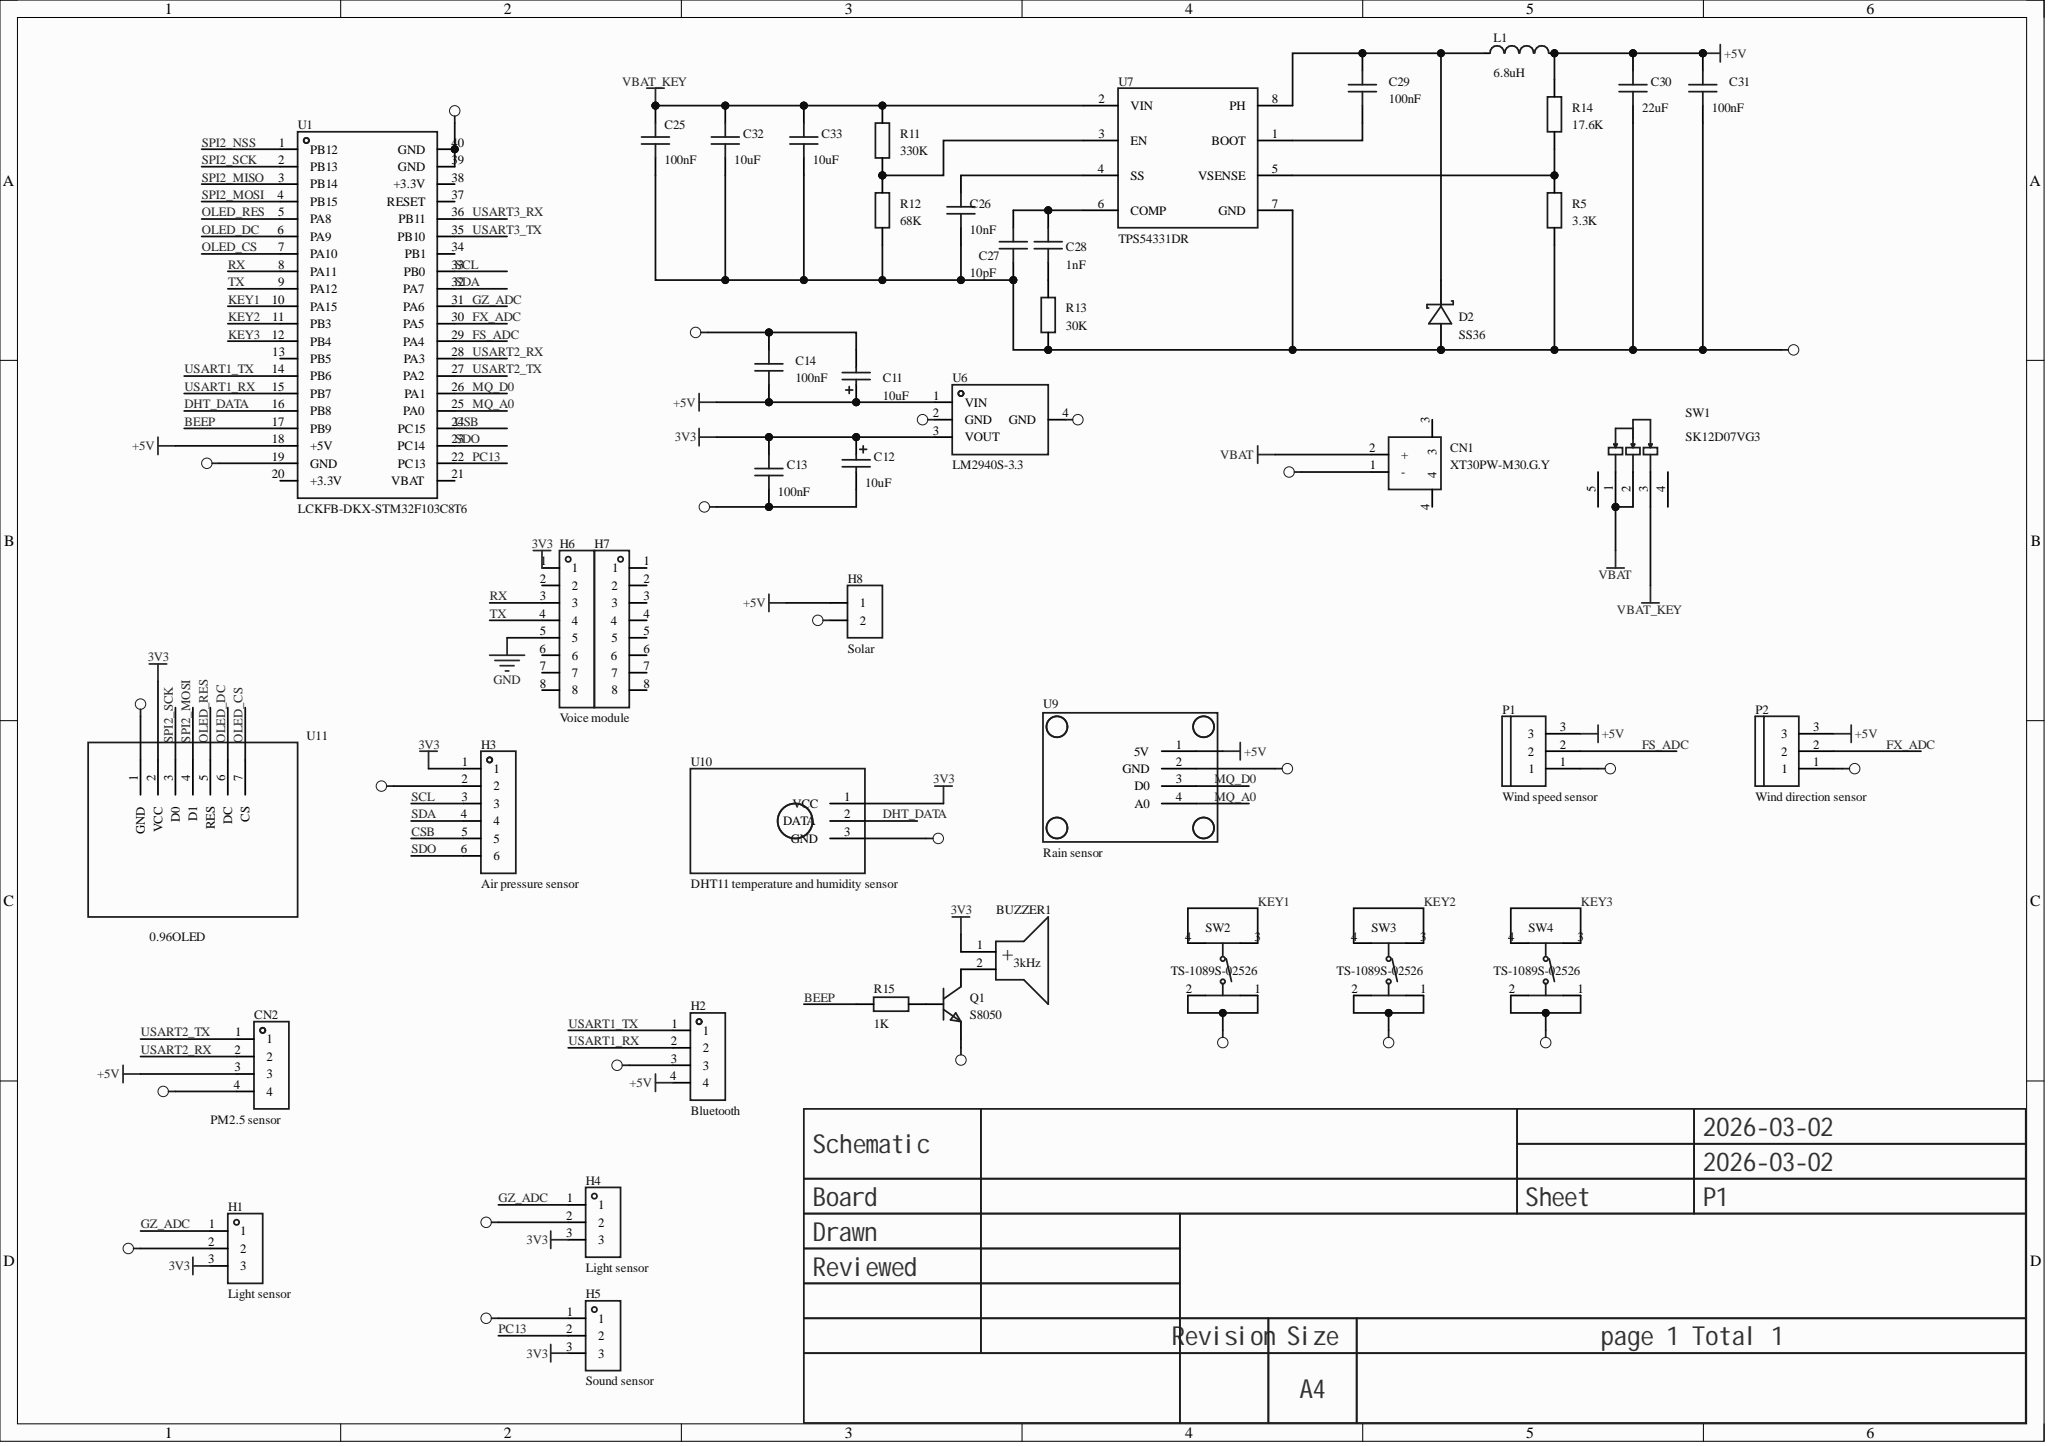Circuit board | Altium Designer | 45 parts | 40 nets
Bill of materials:
Comment,Description,Designator,Footprint,LibRef,Quantity
"3kHz","Drive: active (built-in driver circuit); type: electromagnetic; frequency: 3kHz; SPL: 85dB;","BUZZER1","BUZ-TH_BD9.0-P5.00-D0.6-FD","HNB09A03","1"
"10uF","Capacitance: 10uF; tolerance: ±10%; rated voltage: 10V; ESR: 3O@100kHz;","C11, C12","CASE-A_3216","TAJA106K010RNJ","2"
"100nF","","C13, C14, C25, C29, C31","C0603","CAP_0603","5"
"10nF","","C26","C0603","CAP_0603","1"
"10pF","","C27","C0603","CAP_0603","1"
"1nF","","C28","C0603","CAP_0603","1"
"22uF","","C30","C0603","CAP_0603","1"
"10uF","Capacitance: 10uF; tolerance: ±10%; rated voltage: 50V; dielectric (temperature coefficient): X5R;","C32, C33","C0805","GRM21BR61H106KE43L","2"
"XT30PW-M30.G.Y","Category: -; type 1: -;","CN1","CONN-TH_XT30PW-M","XT30PW-M30.G.Y","1"
"PM2.5 sensor","Pin structure: 1x4P; pitch: 1.5mm; mounting: right angle; reference series: ZH; total PIN count: 4P; rows: 1; PINs per row: 4; row spacing: -; rated current: 1A; contact material: brass; contact plating: tin; operating temperature range: -25℃~+85℃;","CN2","CONN-TH_4P-P1.50_HCTL_HC-ZH1.5-4AW","HC-ZH1.5-4AW","1"
"SS36","Diode configuration: single; forward voltage (Vf): 700mV@3A; DC reverse voltage (Vr): 60V; rectified current: 3A;","D2","SMA_L4.3-W2.6-LS5.2-RD","SS36_C16015","1"
"Light sensor","Socket structure: 1x3P; pitch: 2.54mm; row spacing: -; mounting type: through-hole; rows: single; total holes: 3P; plastic height: -; contact material: brass; contact plating: -;","H1, H4","HDR-TH_3P-P2.54-V-F","PM254V-11-03-H85","2"
"Bluetooth","Socket structure: 1x4P; pitch: 2.54mm; row spacing: -; round/square hole: square hole; mounting type: through-hole; rows: single; total holes: 4P; rated current: 3A; rated voltage: -; socket direction: top; plastic height: -; contact material: bronze; contact plating: -; operating temperature range: -40℃~+105℃; soldering temperature (max): -;","H2","HDR-TH_4P-P2.54-V-F","2.54-1*4P母","1"
"Air pressure sensor","","H3","HDR-TH_6P-P2.54-V-F","HDR-F_2.54_1x6P","1"
"Sound sensor","Socket structure: 1x3P; pitch: 2.54mm; row spacing: -; mounting type: through-hole; rows: single; total holes: 3P; plastic height: -; contact material: brass; contact plating: -;","H5","HDR-TH_3P-P2.54-V-F","PM254V-11-03-H85","1"
"Voice module","","H6","HDR-TH_8P-P2.54-V-F-1","HDR-F_2.54_1x8P","1"
"","","H7","HDR-TH_8P-P2.54-V-F-1","HDR-F_2.54_1x8P","1"
"Solar","","H8","HDR-TH_2P-P2.54-V-F","HDR-F_2.54_1x2P","1"
"6.8uH","Inductance: 6.8uH; tolerance: ±20%; rated current: 5A; saturation current (Isat): 6A; type: molded inductor;","L1","IND-SMD_L7.0-W6.6","FXL0630-6R8-M","1"
"Wind speed sensor","Structure: 1x3P; pitch: 5.08mm; color: green; mounting: through-hole; rated current: 18A; rated voltage: 250V; rows: 1; wire gauge - AWG: 14~30; wire gauge - mm²: 2.5; PINs per row: 3; operating temperature range: -40℃~+105℃;","P1","CONN-TH_3P-P5.00_WJ500V-5.08-3P","WJ500V-5.08-3P","1"
"Wind direction sensor","Structure: 1x3P; pitch: 5.08mm; color: green; mounting: through-hole; rated current: 18A; rated voltage: 250V; rows: 1; wire gauge - AWG: 14~30; wire gauge - mm²: 2.5; PINs per row: 3; operating temperature range: -40℃~+105℃;","P2","CONN-TH_3P-P5.00_WJ500V-5.08-3P","WJ500V-5.08-3P","1"
"S8050","Transistor type: NPN; collector current (Ic): 500mA; collector-emitter breakdown voltage (Vceo): 25V; power dissipation (Pd): 300mW; DC current gain (hFE): 120@50mA,1.0V;","Q1","SOT-23-3_L2.9-W1.3-P1.90-LS2.3-BR","S8050_C20069125","1"
"3.3K","","R5","R0603","Res_0603","1"
"330K","","R11","R0603","Res_0603","1"
"68K","","R12","R0603","Res_0603","1"
"30K","","R13","R0603","Res_0603","1"
"17.6K","","R14","R0603","Res_0603","1"
"1K","","R15","R0603","Res_0603","1"
"SK12D07VG3","Circuit: SPDT; mounting: side entry; switch color: -; rated current (DC): 500mA; rated voltage (DC): 50V; rated current (AC): -; rated voltage (AC): -; mechanical life: 5 thousand cycles;","SW1","SW-TH_SK12D07VG3","SK12D07VG3","1"
"TS-1089S-02526","Circuit: SPST; button shape: oval button; mounting: surface mount; switch length: 4.2mm; switch width: 3.25mm; switch height: 2.5mm; contact current: 50mA; rated voltage (DC): 12V; with light: -; mechanical life: -;","SW2, SW3, SW4","SW-SMD_4P-L4.2-W3.3-P2.15-LS5.1","TS-1089S-02526","3"
"LCKFB-DKX-STM32F103C8T6","","U1","CONN-TH_L53.3-W22.9_STM32F103C8T6-CARD","LCKFB-DKX-STM32F103C8T6","1"
"LM2940S-3.3","Output type: fixed; max input voltage: 30V; output voltage: 3.3V; output current: 1A; PSRR: -; output polarity: positive;","U6","SOT-223-3_L6.5-W3.4-P2.30-LS7.0-BR","LM2940S-3.3","1"
"TPS54331DR","Function type: buck; output type: adjustable; operating voltage: 3.5V~28V; output voltage: -; output current: 3A;","U7","SOIC-8_L5.0-W4.0-P1.27-LS6.0-BL","TPS54331DR","1"
"Rain sensor","","U9","MQ-2烟雾传感器模块","MQ-2烟雾传感器模块","1"
"DHT11 temperature and humidity sensor","","U10","DHT11温湿度模块","DHT11温湿度模块","1"
"0.96OLED","","U11","0.96寸OLED","0.96寸OLED","1"
Netlist (Protel format):
[
BUZZER1
BUZ-TH_BD9.0-P5.00-D0.6-FD
3kHz



]
[
C11
CASE-A_3216
10uF



]
[
C12
CASE-A_3216
10uF



]
[
C13
C0603
100nF



]
[
C14
C0603
100nF



]
[
C25
C0603
100nF



]
[
C26
C0603
10nF



]
[
C27
C0603
10pF



]
[
C28
C0603
1nF



]
[
C29
C0603
100nF



]
[
C30
C0603
22uF



]
[
C31
C0603
100nF



]
[
C32
C0805
10uF



]
[
C33
C0805
10uF



]
[
CN1
CONN-TH_XT30PW-M
XT30PW-M30.G.Y



]
[
CN2
CONN-TH_4P-P1.50_HCTL_HC-ZH1.5-4AW
PM2.5 sensor



]
[
D2
SMA_L4.3-W2.6-LS5.2-RD
SS36



]
[
H1
HDR-TH_3P-P2.54-V-F
Light sensor



]
[
H2
HDR-TH_4P-P2.54-V-F
Bluetooth



]
[
H3
HDR-TH_6P-P2.54-V-F
Air pressure sensor



]
[
H4
HDR-TH_3P-P2.54-V-F
Light sensor



]
[
H5
HDR-TH_3P-P2.54-V-F
Sound sensor



]
[
H6
HDR-TH_8P-P2.54-V-F-1
Voice module



]
[
H7
HDR-TH_8P-P2.54-V-F-1




]
[
H8
HDR-TH_2P-P2.54-V-F
Solar



]
[
L1
IND-SMD_L7.0-W6.6
6.8uH



]
[
P1
CONN-TH_3P-P5.00_WJ500V-5.08-3P
Wind speed sensor



]
[
P2
CONN-TH_3P-P5.00_WJ500V-5.08-3P
Wind direction sensor



]
[
Q1
SOT-23-3_L2.9-W1.3-P1.90-LS2.3-BR
S8050



]
[
R5
R0603
3.3K



]
[
R11
R0603
330K



]
[
R12
R0603
68K



]
[
R13
R0603
30K



]
[
R14
R0603
17.6K



]
[
R15
R0603
1K



]
[
SW1
SW-TH_SK12D07VG3
SK12D07VG3



]
[
SW2
SW-SMD_4P-L4.2-W3.3-P2.15-LS5.1
TS-1089S-02526



]
[
SW3
SW-SMD_4P-L4.2-W3.3-P2.15-LS5.1
TS-1089S-02526



]
[
SW4
SW-SMD_4P-L4.2-W3.3-P2.15-LS5.1
TS-1089S-02526



]
[
U1
CONN-TH_L53.3-W22.9_STM32F103C8T6-CARD
LCKFB-DKX-STM32F103C8T6



]
[
U6
SOT-223-3_L6.5-W3.4-P2.30-LS7.0-BR
LM2940S-3.3



]
[
U7
SOIC-8_L5.0-W4.0-P1.27-LS6.0-BL
TPS54331DR



]
[
U9
MQ-2烟雾传感器模块
Rain sensor



]
[
U10
DHT11温湿度模块
DHT11 temperature and humidity sensor



]
[
U11
0.96寸OLED
0.96OLED



]
(
VBAT_KEY
C25-2
C32-2
C33-2
R11-2
SW1-3
U7-2
)
(
VBAT
CN1-2
SW1-1
SW1-2
)
(
USART2_TX
CN2-1
U1-27
)
(
USART2_RX
CN2-2
U1-28
)
(
USART1_TX
H2-1
U1-14
)
(
USART1_RX
H2-2
U1-15
)
(
TX
H6-4
U1-9
)
(
SPI2_SCK
U1-2
U11-3
)
(
SPI2_MOSI
U1-4
U11-4
)
(
SDO
H3-6
U1-23
)
(
SDA
H3-4
U1-32
)
(
SCL
H3-3
U1-33
)
(
RX
H6-3
U1-8
)
(
PGND
C11-2
C12-2
C13-1
C14-2
C25-1
C26-1
C27-1
C30-1
C31-1
C32-1
C33-1
CN1-1
CN2-4
D2-2
H1-2
H2-3
H3-2
H4-2
H5-1
H8-2
P1-1
P2-1
Q1-2
R5-1
R12-1
R13-1
SW2-1
SW2-2
SW3-1
SW3-2
SW4-1
SW4-2
U1-19
U1-39
U1-40
U6-2
U6-4
U7-7
U9-2
U10-3
U11-1
)
(
PC13
H5-2
U1-22
)
(
OLED_RES
U1-5
U11-5
)
(
OLED_DC
U1-6
U11-6
)
(
OLED_CS
U1-7
U11-7
)
(
NetR11_1
R11-1
R12-2
U7-3
)
(
NetR5_2
R5-2
R14-1
U7-5
)
(
NetQ1_1
Q1-1
R15-2
)
(
NetC29_2
C29-2
D2-1
L1-1
U7-8
)
(
NetC29_1
C29-1
U7-1
)
(
NetC28_1
C28-1
R13-2
)
(
NetC27_2
C27-2
C28-2
U7-6
)
(
NetC26_2
C26-2
U7-4
)
(
NetBUZZER1_2
BUZZER1-2
Q1-3
)
(
MQ_D0
U1-26
U9-3
)
(
MQ_A0
U1-25
U9-4
)
(
KEY3
SW4-3
SW4-4
U1-12
)
(
KEY2
SW3-3
SW3-4
U1-11
)
(
KEY1
SW2-3
SW2-4
U1-10
)
(
GZ_ADC
H1-1
H4-1
U1-31
)
(
FX_ADC
P2-2
U1-30
)
(
FS_ADC
P1-2
U1-29
)
(
DHT_DATA
U1-16
U10-2
)
(
CSB
H3-5
U1-24
)
(
BEEP
R15-1
U1-17
)
(
+5V
C11-1
C14-1
C30-2
C31-2
CN2-3
H2-4
H8-1
L1-2
P1-3
P2-3
R14-2
U1-18
U6-1
U9-1
)
(
3V3
BUZZER1-1
C12-1
C13-2
H1-3
H3-1
H4-3
H5-3
H6-1
U6-3
U10-1
U11-2
)